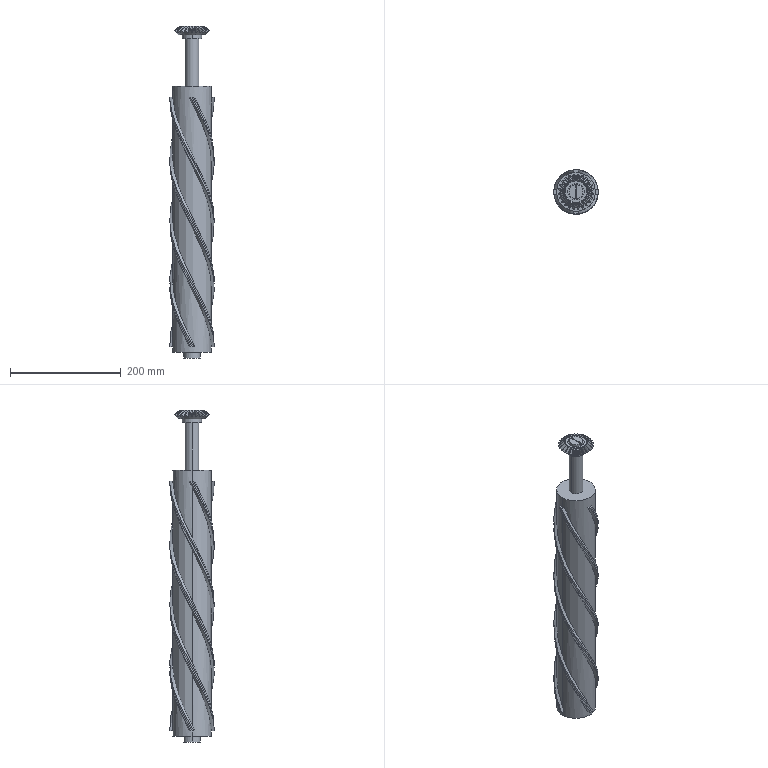Part | SolidWorks | 4 solids | 435 faces | box 80.225 x 80.225 x 598.5 mm | volume 2005498 mm3 | cone 189 | cylinder 113 | spline 88 | plane 33 | torus 10 | sphere 2 | commonest cylinder face diameters 8 x78 70 x8 6 x6 20 x5 0.8 x4 25 x4